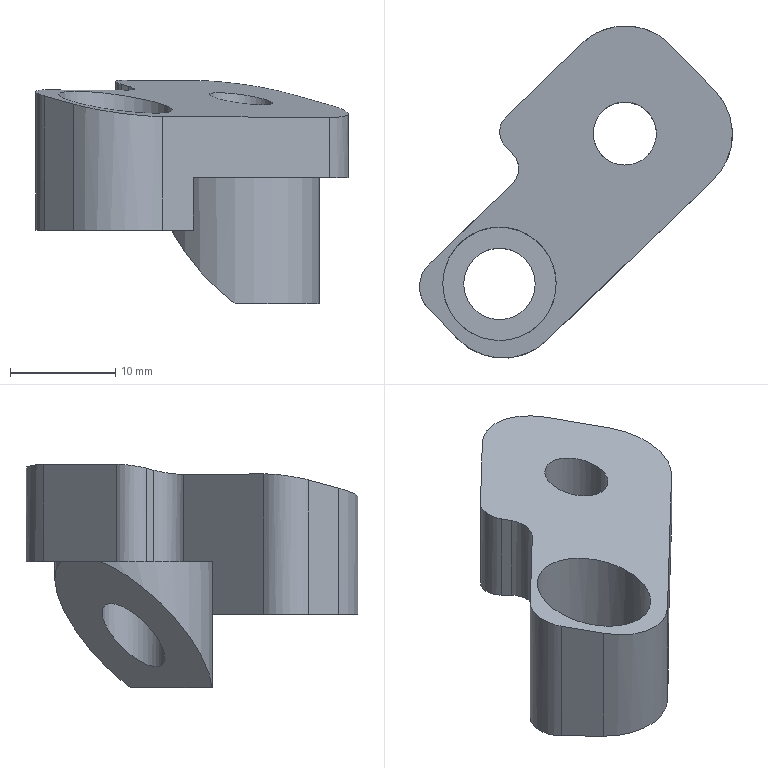Part | STEP file | gslz 2016.10.28-13_id1518_x_t | 1 solid | 25 faces | box 29.762 x 31.599 x 21.259 mm | volume 4382 mm3 | plane 14 | cylinder 10 | spline 1 | commonest cylinder face diameters 12 x3 4 x2 6 x2 6.8 x1 10.8 x1 15 x1